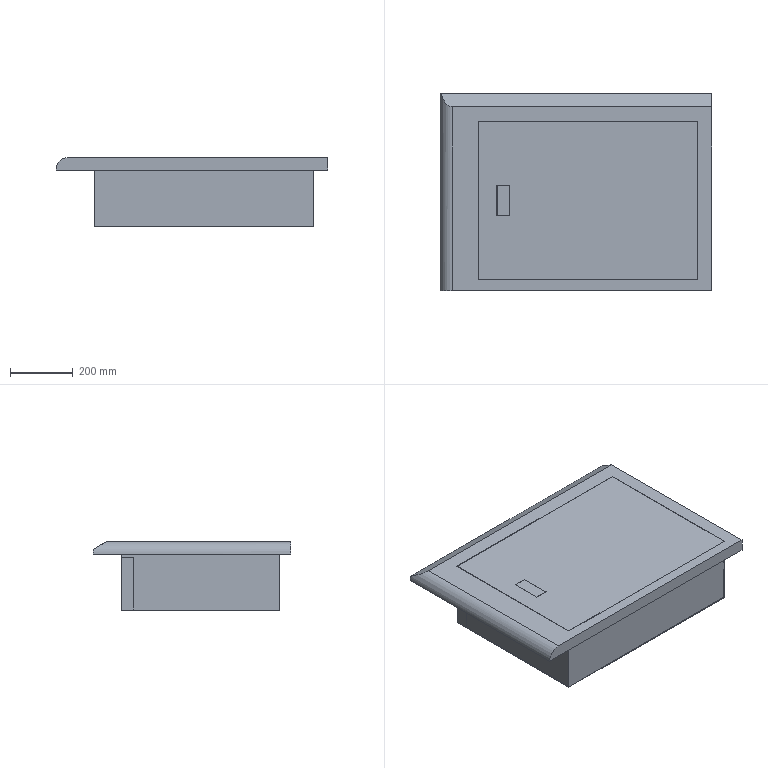Part | SolidWorks | features ICE 9, CutThin 1, Extrusion 1, Fillet 1, Shell 1 | 1 solid | 46 faces | box 867.5 x 630 x 220 mm | volume 27389806 mm3 | plane 45 | cylinder 1 | commonest cylinder face diameters 80 x1
STEP:
#1=CARTESIAN_POINT('',(-122.,595.,180.));
#2=VERTEX_POINT('',#1);
#3=CARTESIAN_POINT('',(-122.,-35.,180.));
#4=VERTEX_POINT('',#3);
#5=CARTESIAN_POINT('',(-122.,595.,180.));
#6=DIRECTION('',(0.,-1.,0.));
#7=VECTOR('',#6,1000.);
#8=LINE('',#5,#7);
#9=EDGE_CURVE('',#2,#4,#8,.T.);
#10=ORIENTED_EDGE('',*,*,#9,.F.);
#11=CARTESIAN_POINT('',(745.5,595.,180.));
#12=VERTEX_POINT('',#11);
#13=CARTESIAN_POINT('',(-122.,595.,180.));
#14=DIRECTION('',(-1.,0.,0.));
#15=VECTOR('',#14,1000.);
#16=LINE('',#13,#15);
#17=EDGE_CURVE('',#12,#2,#16,.T.);
#18=ORIENTED_EDGE('',*,*,#17,.F.);
#19=CARTESIAN_POINT('',(745.5,-35.,180.));
#20=VERTEX_POINT('',#19);
#21=CARTESIAN_POINT('',(745.5,595.,180.));
#22=DIRECTION('',(0.,1.,0.));
#23=VECTOR('',#22,1000.);
#24=LINE('',#21,#23);
#25=EDGE_CURVE('',#20,#12,#24,.T.);
#26=ORIENTED_EDGE('',*,*,#25,.F.);
#27=CARTESIAN_POINT('',(-122.,-35.,180.));
#28=DIRECTION('',(1.,0.,0.));
#29=VECTOR('',#28,1000.);
#30=LINE('',#27,#29);
#31=EDGE_CURVE('',#4,#20,#30,.T.);
#32=ORIENTED_EDGE('',*,*,#31,.F.);
#33=EDGE_LOOP('',(#10,#18,#26,#32));
#34=FACE_OUTER_BOUND('',#33,.T.);
#35=CARTESIAN_POINT('',(700.,505.,180.));
#36=VERTEX_POINT('',#35);
#37=CARTESIAN_POINT('',(0.,505.,180.));
#38=VERTEX_POINT('',#37);
#39=CARTESIAN_POINT('',(0.,505.,180.));
#40=DIRECTION('',(-1.,0.,0.));
#41=VECTOR('',#40,1000.);
#42=LINE('',#39,#41);
#43=EDGE_CURVE('',#36,#38,#42,.T.);
#44=ORIENTED_EDGE('',*,*,#43,.T.);
#45=CARTESIAN_POINT('',(0.,0.,180.));
#46=VERTEX_POINT('',#45);
#47=CARTESIAN_POINT('',(0.,0.,180.));
#48=DIRECTION('',(0.,-1.,0.));
#49=VECTOR('',#48,1000.);
#50=LINE('',#47,#49);
#51=EDGE_CURVE('',#38,#46,#50,.T.);
#52=ORIENTED_EDGE('',*,*,#51,.T.);
#53=CARTESIAN_POINT('',(700.,0.,180.));
#54=VERTEX_POINT('',#53);
#55=CARTESIAN_POINT('',(0.,0.,180.));
#56=DIRECTION('',(1.,0.,0.));
#57=VECTOR('',#56,1000.);
#58=LINE('',#55,#57);
#59=EDGE_CURVE('',#46,#54,#58,.T.);
#60=ORIENTED_EDGE('',*,*,#59,.T.);
#61=CARTESIAN_POINT('',(700.,0.,180.));
#62=DIRECTION('',(0.,1.,0.));
#63=VECTOR('',#62,1000.);
#64=LINE('',#61,#63);
#65=EDGE_CURVE('',#54,#36,#64,.T.);
#66=ORIENTED_EDGE('',*,*,#65,.T.);
#67=EDGE_LOOP('',(#44,#52,#60,#66));
#68=FACE_BOUND('',#67,.T.);
#69=CARTESIAN_POINT('',(0.,0.,180.));
#70=DIRECTION('',(0.,0.,1.));
#71=DIRECTION('',(1.,0.,0.));
#72=AXIS2_PLACEMENT_3D('',#69,#70,#71);
#73=PLANE('',#72);
#74=ADVANCED_FACE('',(#34,#68),#73,.F.);
#75=CARTESIAN_POINT('',(-82.,-35.,220.));
#76=VERTEX_POINT('',#75);
#77=CARTESIAN_POINT('',(745.5,-35.,220.));
#78=VERTEX_POINT('',#77);
#79=CARTESIAN_POINT('',(-122.,-35.,220.));
#80=DIRECTION('',(1.,0.,0.));
#81=VECTOR('',#80,1000.);
#82=LINE('',#79,#81);
#83=EDGE_CURVE('',#76,#78,#82,.T.);
#84=ORIENTED_EDGE('',*,*,#83,.F.);
#85=CARTESIAN_POINT('',(-82.,-35.,180.));
#86=DIRECTION('',(0.,-1.,0.));
#87=DIRECTION('',(0.,0.,1.));
#88=AXIS2_PLACEMENT_3D('',#85,#86,#87);
#89=CIRCLE('',#88,40.);
#90=EDGE_CURVE('',#76,#4,#89,.T.);
#91=ORIENTED_EDGE('',*,*,#90,.T.);
#92=ORIENTED_EDGE('',*,*,#31,.T.);
#93=CARTESIAN_POINT('',(745.5,-35.,220.));
#94=DIRECTION('',(0.,0.,-1.));
#95=VECTOR('',#94,1000.);
#96=LINE('',#93,#95);
#97=EDGE_CURVE('',#78,#20,#96,.T.);
#98=ORIENTED_EDGE('',*,*,#97,.F.);
#99=EDGE_LOOP('',(#84,#91,#92,#98));
#100=FACE_OUTER_BOUND('',#99,.T.);
#101=CARTESIAN_POINT('',(-122.,-35.,220.));
#102=DIRECTION('',(0.,1.,0.));
#103=DIRECTION('',(0.,0.,1.));
#104=AXIS2_PLACEMENT_3D('',#101,#102,#103);
#105=PLANE('',#104);
#106=ADVANCED_FACE('',(#100),#105,.F.);
#107=CARTESIAN_POINT('',(745.5,595.,195.));
#108=VERTEX_POINT('',#107);
#109=CARTESIAN_POINT('',(745.5,595.,220.));
#110=DIRECTION('',(0.,0.,-1.));
#111=VECTOR('',#110,1000.);
#112=LINE('',#109,#111);
#113=EDGE_CURVE('',#108,#12,#112,.T.);
#114=ORIENTED_EDGE('',*,*,#113,.F.);
#115=CARTESIAN_POINT('',(745.5,551.699,220.));
#116=VERTEX_POINT('',#115);
#117=CARTESIAN_POINT('',(745.5,595.,195.));
#118=DIRECTION('',(0.,-0.866,0.5));
#119=VECTOR('',#118,1000.);
#120=LINE('',#117,#119);
#121=EDGE_CURVE('',#108,#116,#120,.T.);
#122=ORIENTED_EDGE('',*,*,#121,.T.);
#123=CARTESIAN_POINT('',(745.5,595.,220.));
#124=DIRECTION('',(0.,1.,0.));
#125=VECTOR('',#124,1000.);
#126=LINE('',#123,#125);
#127=EDGE_CURVE('',#78,#116,#126,.T.);
#128=ORIENTED_EDGE('',*,*,#127,.F.);
#129=ORIENTED_EDGE('',*,*,#97,.T.);
#130=ORIENTED_EDGE('',*,*,#25,.T.);
#131=EDGE_LOOP('',(#114,#122,#128,#129,#130));
#132=FACE_OUTER_BOUND('',#131,.T.);
#133=CARTESIAN_POINT('',(745.5,595.,220.));
#134=DIRECTION('',(-1.,0.,0.));
#135=DIRECTION('',(0.,-1.,0.));
#136=AXIS2_PLACEMENT_3D('',#133,#134,#135);
#137=PLANE('',#136);
#138=ADVANCED_FACE('',(#132),#137,.F.);
#139=ORIENTED_EDGE('',*,*,#17,.T.);
#140=CARTESIAN_POINT('',(-119.081,595.,195.));
#141=VERTEX_POINT('',#140);
#142=CARTESIAN_POINT('',(-82.,595.,180.));
#143=DIRECTION('',(0.,1.,0.));
#144=DIRECTION('',(0.,0.,-1.));
#145=AXIS2_PLACEMENT_3D('',#142,#143,#144);
#146=CIRCLE('',#145,40.);
#147=EDGE_CURVE('',#2,#141,#146,.T.);
#148=ORIENTED_EDGE('',*,*,#147,.T.);
#149=CARTESIAN_POINT('',(745.5,595.,195.));
#150=DIRECTION('',(-1.,0.,0.));
#151=VECTOR('',#150,1000.);
#152=LINE('',#149,#151);
#153=EDGE_CURVE('',#108,#141,#152,.T.);
#154=ORIENTED_EDGE('',*,*,#153,.F.);
#155=ORIENTED_EDGE('',*,*,#113,.T.);
#156=EDGE_LOOP('',(#139,#148,#154,#155));
#157=FACE_OUTER_BOUND('',#156,.T.);
#158=CARTESIAN_POINT('',(-122.,595.,220.));
#159=DIRECTION('',(0.,-1.,0.));
#160=DIRECTION('',(0.,0.,-1.));
#161=AXIS2_PLACEMENT_3D('',#158,#159,#160);
#162=PLANE('',#161);
#163=ADVANCED_FACE('',(#157),#162,.F.);
#164=CARTESIAN_POINT('',(700.5,505.5,220.));
#165=VERTEX_POINT('',#164);
#166=CARTESIAN_POINT('',(-0.5,505.5,220.));
#167=VERTEX_POINT('',#166);
#168=CARTESIAN_POINT('',(700.,505.5,220.));
#169=DIRECTION('',(-1.,0.,0.));
#170=VECTOR('',#169,1000.);
#171=LINE('',#168,#170);
#172=EDGE_CURVE('',#165,#167,#171,.T.);
#173=ORIENTED_EDGE('',*,*,#172,.F.);
#174=CARTESIAN_POINT('',(700.5,-0.5,220.));
#175=VERTEX_POINT('',#174);
#176=CARTESIAN_POINT('',(700.5,0.,220.));
#177=DIRECTION('',(0.,1.,0.));
#178=VECTOR('',#177,1000.);
#179=LINE('',#176,#178);
#180=EDGE_CURVE('',#175,#165,#179,.T.);
#181=ORIENTED_EDGE('',*,*,#180,.F.);
#182=CARTESIAN_POINT('',(-0.5,-0.5,220.));
#183=VERTEX_POINT('',#182);
#184=CARTESIAN_POINT('',(0.,-0.5,220.));
#185=DIRECTION('',(1.,0.,0.));
#186=VECTOR('',#185,1000.);
#187=LINE('',#184,#186);
#188=EDGE_CURVE('',#183,#175,#187,.T.);
#189=ORIENTED_EDGE('',*,*,#188,.F.);
#190=CARTESIAN_POINT('',(-0.5,505.,220.));
#191=DIRECTION('',(0.,-1.,0.));
#192=VECTOR('',#191,1000.);
#193=LINE('',#190,#192);
#194=EDGE_CURVE('',#167,#183,#193,.T.);
#195=ORIENTED_EDGE('',*,*,#194,.F.);
#196=EDGE_LOOP('',(#173,#181,#189,#195));
#197=FACE_BOUND('',#196,.T.);
#198=CARTESIAN_POINT('',(-82.,551.699,220.));
#199=VERTEX_POINT('',#198);
#200=CARTESIAN_POINT('',(745.5,551.699,220.));
#201=DIRECTION('',(-1.,0.,0.));
#202=VECTOR('',#201,1000.);
#203=LINE('',#200,#202);
#204=EDGE_CURVE('',#116,#199,#203,.T.);
#205=ORIENTED_EDGE('',*,*,#204,.T.);
#206=CARTESIAN_POINT('',(-82.,-35.,220.));
#207=DIRECTION('',(0.,-1.,0.));
#208=VECTOR('',#207,1000.);
#209=LINE('',#206,#208);
#210=EDGE_CURVE('',#199,#76,#209,.T.);
#211=ORIENTED_EDGE('',*,*,#210,.T.);
#212=ORIENTED_EDGE('',*,*,#83,.T.);
#213=ORIENTED_EDGE('',*,*,#127,.T.);
#214=EDGE_LOOP('',(#205,#211,#212,#213));
#215=FACE_OUTER_BOUND('',#214,.T.);
#216=CARTESIAN_POINT('',(0.,0.,220.));
#217=DIRECTION('',(0.,0.,1.));
#218=DIRECTION('',(1.,0.,0.));
#219=AXIS2_PLACEMENT_3D('',#216,#217,#218);
#220=PLANE('',#219);
#221=ADVANCED_FACE('',(#197,#215),#220,.T.);
#222=CARTESIAN_POINT('',(0.,505.,0.));
#223=VERTEX_POINT('',#222);
#224=CARTESIAN_POINT('',(0.,0.,0.));
#225=VERTEX_POINT('',#224);
#226=CARTESIAN_POINT('',(0.,0.,0.));
#227=DIRECTION('',(0.,-1.,0.));
#228=VECTOR('',#227,1000.);
#229=LINE('',#226,#228);
#230=EDGE_CURVE('',#223,#225,#229,.T.);
#231=ORIENTED_EDGE('',*,*,#230,.F.);
#232=CARTESIAN_POINT('',(700.,505.,0.));
#233=VERTEX_POINT('',#232);
#234=CARTESIAN_POINT('',(700.,505.,0.));
#235=DIRECTION('',(-1.,0.,0.));
#236=VECTOR('',#235,1000.);
#237=LINE('',#234,#236);
#238=EDGE_CURVE('',#233,#223,#237,.T.);
#239=ORIENTED_EDGE('',*,*,#238,.F.);
#240=CARTESIAN_POINT('',(700.,0.,0.));
#241=VERTEX_POINT('',#240);
#242=CARTESIAN_POINT('',(700.,0.,0.));
#243=DIRECTION('',(0.,1.,0.));
#244=VECTOR('',#243,1000.);
#245=LINE('',#242,#244);
#246=EDGE_CURVE('',#241,#233,#245,.T.);
#247=ORIENTED_EDGE('',*,*,#246,.F.);
#248=CARTESIAN_POINT('',(0.,0.,0.));
#249=DIRECTION('',(1.,0.,0.));
#250=VECTOR('',#249,1000.);
#251=LINE('',#248,#250);
#252=EDGE_CURVE('',#225,#241,#251,.T.);
#253=ORIENTED_EDGE('',*,*,#252,.F.);
#254=EDGE_LOOP('',(#231,#239,#247,#253));
#255=FACE_OUTER_BOUND('',#254,.T.);
#256=CARTESIAN_POINT('',(0.,0.,0.));
#257=DIRECTION('',(0.,0.,-1.));
#258=DIRECTION('',(-1.,0.,0.));
#259=AXIS2_PLACEMENT_3D('',#256,#257,#258);
#260=PLANE('',#259);
#261=ADVANCED_FACE('',(#255),#260,.T.);
#262=CARTESIAN_POINT('',(700.,505.,180.));
#263=DIRECTION('',(0.,0.,-1.));
#264=VECTOR('',#263,1000.);
#265=LINE('',#262,#264);
#266=EDGE_CURVE('',#36,#233,#265,.T.);
#267=ORIENTED_EDGE('',*,*,#266,.T.);
#268=ORIENTED_EDGE('',*,*,#238,.T.);
#269=CARTESIAN_POINT('',(0.,505.,180.));
#270=DIRECTION('',(0.,0.,-1.));
#271=VECTOR('',#270,1000.);
#272=LINE('',#269,#271);
#273=EDGE_CURVE('',#38,#223,#272,.T.);
#274=ORIENTED_EDGE('',*,*,#273,.F.);
#275=ORIENTED_EDGE('',*,*,#43,.F.);
#276=EDGE_LOOP('',(#267,#268,#274,#275));
#277=FACE_OUTER_BOUND('',#276,.T.);
#278=CARTESIAN_POINT('',(0.,505.,180.));
#279=DIRECTION('',(0.,-1.,0.));
#280=DIRECTION('',(0.,0.,-1.));
#281=AXIS2_PLACEMENT_3D('',#278,#279,#280);
#282=PLANE('',#281);
#283=ADVANCED_FACE('',(#277),#282,.F.);
#284=ORIENTED_EDGE('',*,*,#246,.T.);
#285=ORIENTED_EDGE('',*,*,#266,.F.);
#286=ORIENTED_EDGE('',*,*,#65,.F.);
#287=CARTESIAN_POINT('',(700.,0.,180.));
#288=DIRECTION('',(0.,0.,-1.));
#289=VECTOR('',#288,1000.);
#290=LINE('',#287,#289);
#291=EDGE_CURVE('',#54,#241,#290,.T.);
#292=ORIENTED_EDGE('',*,*,#291,.T.);
#293=EDGE_LOOP('',(#284,#285,#286,#292));
#294=FACE_OUTER_BOUND('',#293,.T.);
#295=CARTESIAN_POINT('',(700.,0.,180.));
#296=DIRECTION('',(-1.,0.,0.));
#297=DIRECTION('',(0.,0.,1.));
#298=AXIS2_PLACEMENT_3D('',#295,#296,#297);
#299=PLANE('',#298);
#300=ADVANCED_FACE('',(#294),#299,.F.);
#301=CARTESIAN_POINT('',(0.,0.,180.));
#302=DIRECTION('',(0.,0.,-1.));
#303=VECTOR('',#302,1000.);
#304=LINE('',#301,#303);
#305=EDGE_CURVE('',#46,#225,#304,.T.);
#306=ORIENTED_EDGE('',*,*,#305,.T.);
#307=ORIENTED_EDGE('',*,*,#252,.T.);
#308=ORIENTED_EDGE('',*,*,#291,.F.);
#309=ORIENTED_EDGE('',*,*,#59,.F.);
#310=EDGE_LOOP('',(#306,#307,#308,#309));
#311=FACE_OUTER_BOUND('',#310,.T.);
#312=CARTESIAN_POINT('',(0.,0.,180.));
#313=DIRECTION('',(0.,1.,0.));
#314=DIRECTION('',(0.,0.,1.));
#315=AXIS2_PLACEMENT_3D('',#312,#313,#314);
#316=PLANE('',#315);
#317=ADVANCED_FACE('',(#311),#316,.F.);
#318=ORIENTED_EDGE('',*,*,#273,.T.);
#319=ORIENTED_EDGE('',*,*,#230,.T.);
#320=ORIENTED_EDGE('',*,*,#305,.F.);
#321=ORIENTED_EDGE('',*,*,#51,.F.);
#322=EDGE_LOOP('',(#318,#319,#320,#321));
#323=FACE_OUTER_BOUND('',#322,.T.);
#324=CARTESIAN_POINT('',(0.,0.,180.));
#325=DIRECTION('',(1.,0.,0.));
#326=DIRECTION('',(0.,0.,-1.));
#327=AXIS2_PLACEMENT_3D('',#324,#325,#326);
#328=PLANE('',#327);
#329=ADVANCED_FACE('',(#323),#328,.F.);
#330=ORIENTED_EDGE('',*,*,#153,.T.);
#331=CARTESIAN_POINT('',(-119.081,595.,195.));
#332=CARTESIAN_POINT('',(-112.772,567.988,210.596));
#333=CARTESIAN_POINT('',(-98.823,551.699,220.));
#334=CARTESIAN_POINT('',(-82.,551.699,220.));
#335=(BOUNDED_CURVE()B_SPLINE_CURVE(3,(#331,#332,#333,#334),.UNSPECIFIED.,.F.,.T.)B_SPLINE_CURVE_WITH_KNOTS((4,4),(1.955,3.142),.UNSPECIFIED.)CURVE()GEOMETRIC_REPRESENTATION_ITEM()RATIONAL_B_SPLINE_CURVE((1.,0.8861,0.8861,1.))REPRESENTATION_ITEM(''));
#336=EDGE_CURVE('',#141,#199,#335,.T.);
#337=ORIENTED_EDGE('',*,*,#336,.T.);
#338=ORIENTED_EDGE('',*,*,#204,.F.);
#339=ORIENTED_EDGE('',*,*,#121,.F.);
#340=EDGE_LOOP('',(#330,#337,#338,#339));
#341=FACE_OUTER_BOUND('',#340,.T.);
#342=CARTESIAN_POINT('',(745.5,595.,195.));
#343=DIRECTION('',(0.,-0.5,-0.866));
#344=DIRECTION('',(0.,0.866,-0.5));
#345=AXIS2_PLACEMENT_3D('',#342,#343,#344);
#346=PLANE('',#345);
#347=ADVANCED_FACE('',(#341),#346,.F.);
#348=ORIENTED_EDGE('',*,*,#147,.F.);
#349=ORIENTED_EDGE('',*,*,#9,.T.);
#350=ORIENTED_EDGE('',*,*,#90,.F.);
#351=ORIENTED_EDGE('',*,*,#210,.F.);
#352=ORIENTED_EDGE('',*,*,#336,.F.);
#353=EDGE_LOOP('',(#348,#349,#350,#351,#352));
#354=FACE_OUTER_BOUND('',#353,.T.);
#355=CARTESIAN_POINT('',(-82.,0.,180.));
#356=DIRECTION('',(0.,1.,0.));
#357=DIRECTION('',(-1.,0.,0.));
#358=AXIS2_PLACEMENT_3D('',#355,#356,#357);
#359=CYLINDRICAL_SURFACE('',#358,40.);
#360=ADVANCED_FACE('',(#354),#359,.T.);
#361=ORIENTED_EDGE('',*,*,#172,.T.);
#362=CARTESIAN_POINT('',(-0.5,505.5,210.));
#363=VERTEX_POINT('',#362);
#364=CARTESIAN_POINT('',(-0.5,505.5,210.));
#365=DIRECTION('',(0.,0.,1.));
#366=VECTOR('',#365,1000.);
#367=LINE('',#364,#366);
#368=EDGE_CURVE('',#363,#167,#367,.T.);
#369=ORIENTED_EDGE('',*,*,#368,.F.);
#370=CARTESIAN_POINT('',(700.5,505.5,210.));
#371=VERTEX_POINT('',#370);
#372=CARTESIAN_POINT('',(700.,505.5,210.));
#373=DIRECTION('',(-1.,0.,0.));
#374=VECTOR('',#373,1000.);
#375=LINE('',#372,#374);
#376=EDGE_CURVE('',#371,#363,#375,.T.);
#377=ORIENTED_EDGE('',*,*,#376,.F.);
#378=CARTESIAN_POINT('',(700.5,505.5,210.));
#379=DIRECTION('',(0.,0.,1.));
#380=VECTOR('',#379,1000.);
#381=LINE('',#378,#380);
#382=EDGE_CURVE('',#371,#165,#381,.T.);
#383=ORIENTED_EDGE('',*,*,#382,.T.);
#384=EDGE_LOOP('',(#361,#369,#377,#383));
#385=FACE_OUTER_BOUND('',#384,.T.);
#386=CARTESIAN_POINT('',(700.,505.5,210.));
#387=DIRECTION('',(0.,1.,0.));
#388=DIRECTION('',(0.,0.,1.));
#389=AXIS2_PLACEMENT_3D('',#386,#387,#388);
#390=PLANE('',#389);
#391=ADVANCED_FACE('',(#385),#390,.F.);
#392=ORIENTED_EDGE('',*,*,#180,.T.);
#393=ORIENTED_EDGE('',*,*,#382,.F.);
#394=CARTESIAN_POINT('',(700.5,-0.5,210.));
#395=VERTEX_POINT('',#394);
#396=CARTESIAN_POINT('',(700.5,0.,210.));
#397=DIRECTION('',(0.,1.,0.));
#398=VECTOR('',#397,1000.);
#399=LINE('',#396,#398);
#400=EDGE_CURVE('',#395,#371,#399,.T.);
#401=ORIENTED_EDGE('',*,*,#400,.F.);
#402=CARTESIAN_POINT('',(700.5,-0.5,210.));
#403=DIRECTION('',(0.,0.,1.));
#404=VECTOR('',#403,1000.);
#405=LINE('',#402,#404);
#406=EDGE_CURVE('',#395,#175,#405,.T.);
#407=ORIENTED_EDGE('',*,*,#406,.T.);
#408=EDGE_LOOP('',(#392,#393,#401,#407));
#409=FACE_OUTER_BOUND('',#408,.T.);
#410=CARTESIAN_POINT('',(700.5,0.,210.));
#411=DIRECTION('',(1.,0.,0.));
#412=DIRECTION('',(0.,0.,-1.));
#413=AXIS2_PLACEMENT_3D('',#410,#411,#412);
#414=PLANE('',#413);
#415=ADVANCED_FACE('',(#409),#414,.F.);
#416=ORIENTED_EDGE('',*,*,#188,.T.);
#417=ORIENTED_EDGE('',*,*,#406,.F.);
#418=CARTESIAN_POINT('',(-0.5,-0.5,210.));
#419=VERTEX_POINT('',#418);
#420=CARTESIAN_POINT('',(0.,-0.5,210.));
#421=DIRECTION('',(1.,0.,0.));
#422=VECTOR('',#421,1000.);
#423=LINE('',#420,#422);
#424=EDGE_CURVE('',#419,#395,#423,.T.);
#425=ORIENTED_EDGE('',*,*,#424,.F.);
#426=CARTESIAN_POINT('',(-0.5,-0.5,210.));
#427=DIRECTION('',(0.,0.,1.));
#428=VECTOR('',#427,1000.);
#429=LINE('',#426,#428);
#430=EDGE_CURVE('',#419,#183,#429,.T.);
#431=ORIENTED_EDGE('',*,*,#430,.T.);
#432=EDGE_LOOP('',(#416,#417,#425,#431));
#433=FACE_OUTER_BOUND('',#432,.T.);
#434=CARTESIAN_POINT('',(0.,-0.5,210.));
#435=DIRECTION('',(0.,-1.,0.));
#436=DIRECTION('',(0.,0.,-1.));
#437=AXIS2_PLACEMENT_3D('',#434,#435,#436);
#438=PLANE('',#437);
#439=ADVANCED_FACE('',(#433),#438,.F.);
#440=ORIENTED_EDGE('',*,*,#194,.T.);
#441=ORIENTED_EDGE('',*,*,#430,.F.);
#442=CARTESIAN_POINT('',(-0.5,505.,210.));
#443=DIRECTION('',(0.,-1.,0.));
#444=VECTOR('',#443,1000.);
#445=LINE('',#442,#444);
#446=EDGE_CURVE('',#363,#419,#445,.T.);
#447=ORIENTED_EDGE('',*,*,#446,.F.);
#448=ORIENTED_EDGE('',*,*,#368,.T.);
#449=EDGE_LOOP('',(#440,#441,#447,#448));
#450=FACE_OUTER_BOUND('',#449,.T.);
#451=CARTESIAN_POINT('',(-0.5,505.,210.));
#452=DIRECTION('',(-1.,0.,0.));
#453=DIRECTION('',(0.,0.,1.));
#454=AXIS2_PLACEMENT_3D('',#451,#452,#453);
#455=PLANE('',#454);
#456=ADVANCED_FACE('',(#450),#455,.F.);
#457=CARTESIAN_POINT('',(700.,0.,210.));
#458=VERTEX_POINT('',#457);
#459=CARTESIAN_POINT('',(700.,505.,210.));
#460=VERTEX_POINT('',#459);
#461=CARTESIAN_POINT('',(700.,0.,210.));
#462=DIRECTION('',(0.,1.,0.));
#463=VECTOR('',#462,1000.);
#464=LINE('',#461,#463);
#465=EDGE_CURVE('',#458,#460,#464,.T.);
#466=ORIENTED_EDGE('',*,*,#465,.F.);
#467=CARTESIAN_POINT('',(0.,0.,210.));
#468=VERTEX_POINT('',#467);
#469=CARTESIAN_POINT('',(0.,0.,210.));
#470=DIRECTION('',(1.,0.,0.));
#471=VECTOR('',#470,1000.);
#472=LINE('',#469,#471);
#473=EDGE_CURVE('',#468,#458,#472,.T.);
#474=ORIENTED_EDGE('',*,*,#473,.F.);
#475=CARTESIAN_POINT('',(0.,505.,210.));
#476=VERTEX_POINT('',#475);
#477=CARTESIAN_POINT('',(0.,505.,210.));
#478=DIRECTION('',(0.,-1.,0.));
#479=VECTOR('',#478,1000.);
#480=LINE('',#477,#479);
#481=EDGE_CURVE('',#476,#468,#480,.T.);
#482=ORIENTED_EDGE('',*,*,#481,.F.);
#483=CARTESIAN_POINT('',(700.,505.,210.));
#484=DIRECTION('',(-1.,0.,0.));
#485=VECTOR('',#484,1000.);
#486=LINE('',#483,#485);
#487=EDGE_CURVE('',#460,#476,#486,.T.);
#488=ORIENTED_EDGE('',*,*,#487,.F.);
#489=EDGE_LOOP('',(#466,#474,#482,#488));
#490=FACE_BOUND('',#489,.T.);
#491=ORIENTED_EDGE('',*,*,#376,.T.);
#492=ORIENTED_EDGE('',*,*,#446,.T.);
#493=ORIENTED_EDGE('',*,*,#424,.T.);
#494=ORIENTED_EDGE('',*,*,#400,.T.);
#495=EDGE_LOOP('',(#491,#492,#493,#494));
#496=FACE_OUTER_BOUND('',#495,.T.);
#497=CARTESIAN_POINT('',(0.,0.,210.));
#498=DIRECTION('',(0.,0.,1.));
#499=DIRECTION('',(1.,0.,0.));
#500=AXIS2_PLACEMENT_3D('',#497,#498,#499);
#501=PLANE('',#500);
#502=ADVANCED_FACE('',(#490,#496),#501,.T.);
#503=CARTESIAN_POINT('',(700.,505.,220.));
#504=VERTEX_POINT('',#503);
#505=CARTESIAN_POINT('',(0.,505.,220.));
#506=VERTEX_POINT('',#505);
#507=CARTESIAN_POINT('',(700.,505.,220.));
#508=DIRECTION('',(-1.,0.,0.));
#509=VECTOR('',#508,1000.);
#510=LINE('',#507,#509);
#511=EDGE_CURVE('',#504,#506,#510,.T.);
#512=ORIENTED_EDGE('',*,*,#511,.F.);
#513=CARTESIAN_POINT('',(700.,505.,210.));
#514=DIRECTION('',(0.,0.,1.));
#515=VECTOR('',#514,1000.);
#516=LINE('',#513,#515);
#517=EDGE_CURVE('',#460,#504,#516,.T.);
#518=ORIENTED_EDGE('',*,*,#517,.F.);
#519=ORIENTED_EDGE('',*,*,#487,.T.);
#520=CARTESIAN_POINT('',(0.,505.,210.));
#521=DIRECTION('',(0.,0.,1.));
#522=VECTOR('',#521,1000.);
#523=LINE('',#520,#522);
#524=EDGE_CURVE('',#476,#506,#523,.T.);
#525=ORIENTED_EDGE('',*,*,#524,.T.);
#526=EDGE_LOOP('',(#512,#518,#519,#525));
#527=FACE_OUTER_BOUND('',#526,.T.);
#528=CARTESIAN_POINT('',(700.,505.,210.));
#529=DIRECTION('',(0.,1.,0.));
#530=DIRECTION('',(0.,0.,1.));
#531=AXIS2_PLACEMENT_3D('',#528,#529,#530);
#532=PLANE('',#531);
#533=ADVANCED_FACE('',(#527),#532,.T.);
#534=CARTESIAN_POINT('',(700.,0.,220.));
#535=VERTEX_POINT('',#534);
#536=CARTESIAN_POINT('',(700.,0.,220.));
#537=DIRECTION('',(0.,1.,0.));
#538=VECTOR('',#537,1000.);
#539=LINE('',#536,#538);
#540=EDGE_CURVE('',#535,#504,#539,.T.);
#541=ORIENTED_EDGE('',*,*,#540,.F.);
#542=CARTESIAN_POINT('',(700.,0.,210.));
#543=DIRECTION('',(0.,0.,1.));
#544=VECTOR('',#543,1000.);
#545=LINE('',#542,#544);
#546=EDGE_CURVE('',#458,#535,#545,.T.);
#547=ORIENTED_EDGE('',*,*,#546,.F.);
#548=ORIENTED_EDGE('',*,*,#465,.T.);
#549=ORIENTED_EDGE('',*,*,#517,.T.);
#550=EDGE_LOOP('',(#541,#547,#548,#549));
#551=FACE_OUTER_BOUND('',#550,.T.);
#552=CARTESIAN_POINT('',(700.,0.,210.));
#553=DIRECTION('',(1.,0.,0.));
#554=DIRECTION('',(0.,0.,-1.));
#555=AXIS2_PLACEMENT_3D('',#552,#553,#554);
#556=PLANE('',#555);
#557=ADVANCED_FACE('',(#551),#556,.T.);
#558=CARTESIAN_POINT('',(0.,0.,220.));
#559=VERTEX_POINT('',#558);
#560=CARTESIAN_POINT('',(0.,0.,220.));
#561=DIRECTION('',(1.,0.,0.));
#562=VECTOR('',#561,1000.);
#563=LINE('',#560,#562);
#564=EDGE_CURVE('',#559,#535,#563,.T.);
#565=ORIENTED_EDGE('',*,*,#564,.F.);
#566=CARTESIAN_POINT('',(0.,0.,210.));
#567=DIRECTION('',(0.,0.,1.));
#568=VECTOR('',#567,1000.);
#569=LINE('',#566,#568);
#570=EDGE_CURVE('',#468,#559,#569,.T.);
#571=ORIENTED_EDGE('',*,*,#570,.F.);
#572=ORIENTED_EDGE('',*,*,#473,.T.);
#573=ORIENTED_EDGE('',*,*,#546,.T.);
#574=EDGE_LOOP('',(#565,#571,#572,#573));
#575=FACE_OUTER_BOUND('',#574,.T.);
#576=CARTESIAN_POINT('',(0.,0.,210.));
#577=DIRECTION('',(0.,-1.,0.));
#578=DIRECTION('',(0.,0.,-1.));
#579=AXIS2_PLACEMENT_3D('',#576,#577,#578);
#580=PLANE('',#579);
#581=ADVANCED_FACE('',(#575),#580,.T.);
#582=CARTESIAN_POINT('',(0.,505.,220.));
#583=DIRECTION('',(0.,-1.,0.));
#584=VECTOR('',#583,1000.);
#585=LINE('',#582,#584);
#586=EDGE_CURVE('',#506,#559,#585,.T.);
#587=ORIENTED_EDGE('',*,*,#586,.F.);
#588=ORIENTED_EDGE('',*,*,#524,.F.);
#589=ORIENTED_EDGE('',*,*,#481,.T.);
#590=ORIENTED_EDGE('',*,*,#570,.T.);
#591=EDGE_LOOP('',(#587,#588,#589,#590));
#592=FACE_OUTER_BOUND('',#591,.T.);
#593=CARTESIAN_POINT('',(0.,505.,210.));
#594=DIRECTION('',(-1.,0.,0.));
#595=DIRECTION('',(0.,0.,1.));
#596=AXIS2_PLACEMENT_3D('',#593,#594,#595);
#597=PLANE('',#596);
#598=ADVANCED_FACE('',(#592),#597,.T.);
#599=CARTESIAN_POINT('',(59.5,301.,220.));
#600=VERTEX_POINT('',#599);
#601=CARTESIAN_POINT('',(59.5,204.,220.));
#602=VERTEX_POINT('',#601);
#603=CARTESIAN_POINT('',(59.5,300.5,220.));
#604=DIRECTION('',(0.,-1.,0.));
#605=VECTOR('',#604,1000.);
#606=LINE('',#603,#605);
#607=EDGE_CURVE('',#600,#602,#606,.T.);
#608=ORIENTED_EDGE('',*,*,#607,.F.);
#609=CARTESIAN_POINT('',(100.5,301.,220.));
#610=VERTEX_POINT('',#609);
#611=CARTESIAN_POINT('',(60.,301.,220.));
#612=DIRECTION('',(-1.,0.,0.));
#613=VECTOR('',#612,1000.);
#614=LINE('',#611,#613);
#615=EDGE_CURVE('',#610,#600,#614,.T.);
#616=ORIENTED_EDGE('',*,*,#615,.F.);
#617=CARTESIAN_POINT('',(100.5,204.,220.));
#618=VERTEX_POINT('',#617);
#619=CARTESIAN_POINT('',(100.5,300.5,220.));
#620=DIRECTION('',(0.,1.,0.));
#621=VECTOR('',#620,1000.);
#622=LINE('',#619,#621);
#623=EDGE_CURVE('',#618,#610,#622,.T.);
#624=ORIENTED_EDGE('',*,*,#623,.F.);
#625=CARTESIAN_POINT('',(60.,204.,220.));
#626=DIRECTION('',(1.,0.,0.));
#627=VECTOR('',#626,1000.);
#628=LINE('',#625,#627);
#629=EDGE_CURVE('',#602,#618,#628,.T.);
#630=ORIENTED_EDGE('',*,*,#629,.F.);
#631=EDGE_LOOP('',(#608,#616,#624,#630));
#632=FACE_BOUND('',#631,.T.);
#633=ORIENTED_EDGE('',*,*,#540,.T.);
#634=ORIENTED_EDGE('',*,*,#511,.T.);
#635=ORIENTED_EDGE('',*,*,#586,.T.);
#636=ORIENTED_EDGE('',*,*,#564,.T.);
#637=EDGE_LOOP('',(#633,#634,#635,#636));
#638=FACE_OUTER_BOUND('',#637,.T.);
#639=CARTESIAN_POINT('',(0.,0.,220.));
#640=DIRECTION('',(0.,0.,1.));
#641=DIRECTION('',(1.,0.,0.));
#642=AXIS2_PLACEMENT_3D('',#639,#640,#641);
#643=PLANE('',#642);
#644=ADVANCED_FACE('',(#632,#638),#643,.T.);
#645=ORIENTED_EDGE('',*,*,#607,.T.);
#646=CARTESIAN_POINT('',(59.5,204.,210.));
#647=VERTEX_POINT('',#646);
#648=CARTESIAN_POINT('',(59.5,204.,210.));
#649=DIRECTION('',(0.,0.,1.));
#650=VECTOR('',#649,1000.);
#651=LINE('',#648,#650);
#652=EDGE_CURVE('',#647,#602,#651,.T.);
#653=ORIENTED_EDGE('',*,*,#652,.F.);
#654=CARTESIAN_POINT('',(59.5,301.,210.));
#655=VERTEX_POINT('',#654);
#656=CARTESIAN_POINT('',(59.5,300.5,210.));
#657=DIRECTION('',(0.,-1.,0.));
#658=VECTOR('',#657,1000.);
#659=LINE('',#656,#658);
#660=EDGE_CURVE('',#655,#647,#659,.T.);
#661=ORIENTED_EDGE('',*,*,#660,.F.);
#662=CARTESIAN_POINT('',(59.5,301.,210.));
#663=DIRECTION('',(0.,0.,1.));
#664=VECTOR('',#663,1000.);
#665=LINE('',#662,#664);
#666=EDGE_CURVE('',#655,#600,#665,.T.);
#667=ORIENTED_EDGE('',*,*,#666,.T.);
#668=EDGE_LOOP('',(#645,#653,#661,#667));
#669=FACE_OUTER_BOUND('',#668,.T.);
#670=CARTESIAN_POINT('',(59.5,300.5,210.));
#671=DIRECTION('',(-1.,0.,0.));
#672=DIRECTION('',(0.,0.,1.));
#673=AXIS2_PLACEMENT_3D('',#670,#671,#672);
#674=PLANE('',#673);
#675=ADVANCED_FACE('',(#669),#674,.F.);
#676=ORIENTED_EDGE('',*,*,#615,.T.);
#677=ORIENTED_EDGE('',*,*,#666,.F.);
#678=CARTESIAN_POINT('',(100.5,301.,210.));
#679=VERTEX_POINT('',#678);
#680=CARTESIAN_POINT('',(60.,301.,210.));
#681=DIRECTION('',(-1.,0.,0.));
#682=VECTOR('',#681,1000.);
#683=LINE('',#680,#682);
#684=EDGE_CURVE('',#679,#655,#683,.T.);
#685=ORIENTED_EDGE('',*,*,#684,.F.);
#686=CARTESIAN_POINT('',(100.5,301.,210.));
#687=DIRECTION('',(0.,0.,1.));
#688=VECTOR('',#687,1000.);
#689=LINE('',#686,#688);
#690=EDGE_CURVE('',#679,#610,#689,.T.);
#691=ORIENTED_EDGE('',*,*,#690,.T.);
#692=EDGE_LOOP('',(#676,#677,#685,#691));
#693=FACE_OUTER_BOUND('',#692,.T.);
#694=CARTESIAN_POINT('',(60.,301.,210.));
#695=DIRECTION('',(0.,1.,0.));
#696=DIRECTION('',(0.,0.,1.));
#697=AXIS2_PLACEMENT_3D('',#694,#695,#696);
#698=PLANE('',#697);
#699=ADVANCED_FACE('',(#693),#698,.F.);
#700=ORIENTED_EDGE('',*,*,#623,.T.);
#701=ORIENTED_EDGE('',*,*,#690,.F.);
#702=CARTESIAN_POINT('',(100.5,204.,210.));
#703=VERTEX_POINT('',#702);
#704=CARTESIAN_POINT('',(100.5,300.5,210.));
#705=DIRECTION('',(0.,1.,0.));
#706=VECTOR('',#705,1000.);
#707=LINE('',#704,#706);
#708=EDGE_CURVE('',#703,#679,#707,.T.);
#709=ORIENTED_EDGE('',*,*,#708,.F.);
#710=CARTESIAN_POINT('',(100.5,204.,210.));
#711=DIRECTION('',(0.,0.,1.));
#712=VECTOR('',#711,1000.);
#713=LINE('',#710,#712);
#714=EDGE_CURVE('',#703,#618,#713,.T.);
#715=ORIENTED_EDGE('',*,*,#714,.T.);
#716=EDGE_LOOP('',(#700,#701,#709,#715));
#717=FACE_OUTER_BOUND('',#716,.T.);
#718=CARTESIAN_POINT('',(100.5,300.5,210.));
#719=DIRECTION('',(1.,0.,0.));
#720=DIRECTION('',(0.,0.,-1.));
#721=AXIS2_PLACEMENT_3D('',#718,#719,#720);
#722=PLANE('',#721);
#723=ADVANCED_FACE('',(#717),#722,.F.);
#724=ORIENTED_EDGE('',*,*,#629,.T.);
#725=ORIENTED_EDGE('',*,*,#714,.F.);
#726=CARTESIAN_POINT('',(60.,204.,210.));
#727=DIRECTION('',(1.,0.,0.));
#728=VECTOR('',#727,1000.);
#729=LINE('',#726,#728);
#730=EDGE_CURVE('',#647,#703,#729,.T.);
#731=ORIENTED_EDGE('',*,*,#730,.F.);
#732=ORIENTED_EDGE('',*,*,#652,.T.);
#733=EDGE_LOOP('',(#724,#725,#731,#732));
#734=FACE_OUTER_BOUND('',#733,.T.);
#735=CARTESIAN_POINT('',(60.,204.,210.));
#736=DIRECTION('',(0.,-1.,0.));
#737=DIRECTION('',(0.,0.,-1.));
#738=AXIS2_PLACEMENT_3D('',#735,#736,#737);
#739=PLANE('',#738);
#740=ADVANCED_FACE('',(#734),#739,.F.);
#741=CARTESIAN_POINT('',(100.,300.5,210.));
#742=VERTEX_POINT('',#741);
#743=CARTESIAN_POINT('',(60.,300.5,210.));
#744=VERTEX_POINT('',#743);
#745=CARTESIAN_POINT('',(60.,300.5,210.));
#746=DIRECTION('',(-1.,0.,0.));
#747=VECTOR('',#746,1000.);
#748=LINE('',#745,#747);
#749=EDGE_CURVE('',#742,#744,#748,.T.);
#750=ORIENTED_EDGE('',*,*,#749,.F.);
#751=CARTESIAN_POINT('',(100.,204.5,210.));
#752=VERTEX_POINT('',#751);
#753=CARTESIAN_POINT('',(100.,300.5,210.));
#754=DIRECTION('',(0.,1.,0.));
#755=VECTOR('',#754,1000.);
#756=LINE('',#753,#755);
#757=EDGE_CURVE('',#752,#742,#756,.T.);
#758=ORIENTED_EDGE('',*,*,#757,.F.);
#759=CARTESIAN_POINT('',(60.,204.5,210.));
#760=VERTEX_POINT('',#759);
#761=CARTESIAN_POINT('',(60.,204.5,210.));
#762=DIRECTION('',(1.,0.,0.));
#763=VECTOR('',#762,1000.);
#764=LINE('',#761,#763);
#765=EDGE_CURVE('',#760,#752,#764,.T.);
#766=ORIENTED_EDGE('',*,*,#765,.F.);
#767=CARTESIAN_POINT('',(60.,300.5,210.));
#768=DIRECTION('',(0.,-1.,0.));
#769=VECTOR('',#768,1000.);
#770=LINE('',#767,#769);
#771=EDGE_CURVE('',#744,#760,#770,.T.);
#772=ORIENTED_EDGE('',*,*,#771,.F.);
#773=EDGE_LOOP('',(#750,#758,#766,#772));
#774=FACE_BOUND('',#773,.T.);
#775=ORIENTED_EDGE('',*,*,#660,.T.);
#776=ORIENTED_EDGE('',*,*,#730,.T.);
#777=ORIENTED_EDGE('',*,*,#708,.T.);
#778=ORIENTED_EDGE('',*,*,#684,.T.);
#779=EDGE_LOOP('',(#775,#776,#777,#778));
#780=FACE_OUTER_BOUND('',#779,.T.);
#781=CARTESIAN_POINT('',(0.,0.,210.));
#782=DIRECTION('',(0.,0.,1.));
#783=DIRECTION('',(1.,0.,0.));
#784=AXIS2_PLACEMENT_3D('',#781,#782,#783);
#785=PLANE('',#784);
#786=ADVANCED_FACE('',(#774,#780),#785,.T.);
#787=CARTESIAN_POINT('',(60.,300.5,220.));
#788=VERTEX_POINT('',#787);
#789=CARTESIAN_POINT('',(60.,204.5,220.));
#790=VERTEX_POINT('',#789);
#791=CARTESIAN_POINT('',(60.,300.5,220.));
#792=DIRECTION('',(0.,-1.,0.));
#793=VECTOR('',#792,1000.);
#794=LINE('',#791,#793);
#795=EDGE_CURVE('',#788,#790,#794,.T.);
#796=ORIENTED_EDGE('',*,*,#795,.F.);
#797=CARTESIAN_POINT('',(60.,300.5,210.));
#798=DIRECTION('',(0.,0.,1.));
#799=VECTOR('',#798,1000.);
#800=LINE('',#797,#799);
#801=EDGE_CURVE('',#744,#788,#800,.T.);
#802=ORIENTED_EDGE('',*,*,#801,.F.);
#803=ORIENTED_EDGE('',*,*,#771,.T.);
#804=CARTESIAN_POINT('',(60.,204.5,210.));
#805=DIRECTION('',(0.,0.,1.));
#806=VECTOR('',#805,1000.);
#807=LINE('',#804,#806);
#808=EDGE_CURVE('',#760,#790,#807,.T.);
#809=ORIENTED_EDGE('',*,*,#808,.T.);
#810=EDGE_LOOP('',(#796,#802,#803,#809));
#811=FACE_OUTER_BOUND('',#810,.T.);
#812=CARTESIAN_POINT('',(60.,300.5,210.));
#813=DIRECTION('',(-1.,0.,0.));
#814=DIRECTION('',(0.,0.,1.));
#815=AXIS2_PLACEMENT_3D('',#812,#813,#814);
#816=PLANE('',#815);
#817=ADVANCED_FACE('',(#811),#816,.T.);
#818=CARTESIAN_POINT('',(100.,300.5,220.));
#819=VERTEX_POINT('',#818);
#820=CARTESIAN_POINT('',(60.,300.5,220.));
#821=DIRECTION('',(-1.,0.,0.));
#822=VECTOR('',#821,1000.);
#823=LINE('',#820,#822);
#824=EDGE_CURVE('',#819,#788,#823,.T.);
#825=ORIENTED_EDGE('',*,*,#824,.F.);
#826=CARTESIAN_POINT('',(100.,300.5,210.));
#827=DIRECTION('',(0.,0.,1.));
#828=VECTOR('',#827,1000.);
#829=LINE('',#826,#828);
#830=EDGE_CURVE('',#742,#819,#829,.T.);
#831=ORIENTED_EDGE('',*,*,#830,.F.);
#832=ORIENTED_EDGE('',*,*,#749,.T.);
#833=ORIENTED_EDGE('',*,*,#801,.T.);
#834=EDGE_LOOP('',(#825,#831,#832,#833));
#835=FACE_OUTER_BOUND('',#834,.T.);
#836=CARTESIAN_POINT('',(60.,300.5,210.));
#837=DIRECTION('',(0.,1.,0.));
#838=DIRECTION('',(0.,0.,1.));
#839=AXIS2_PLACEMENT_3D('',#836,#837,#838);
#840=PLANE('',#839);
#841=ADVANCED_FACE('',(#835),#840,.T.);
#842=CARTESIAN_POINT('',(100.,204.5,220.));
#843=VERTEX_POINT('',#842);
#844=CARTESIAN_POINT('',(100.,300.5,220.));
#845=DIRECTION('',(0.,1.,0.));
#846=VECTOR('',#845,1000.);
#847=LINE('',#844,#846);
#848=EDGE_CURVE('',#843,#819,#847,.T.);
#849=ORIENTED_EDGE('',*,*,#848,.F.);
#850=CARTESIAN_POINT('',(100.,204.5,210.));
#851=DIRECTION('',(0.,0.,1.));
#852=VECTOR('',#851,1000.);
#853=LINE('',#850,#852);
#854=EDGE_CURVE('',#752,#843,#853,.T.);
#855=ORIENTED_EDGE('',*,*,#854,.F.);
#856=ORIENTED_EDGE('',*,*,#757,.T.);
#857=ORIENTED_EDGE('',*,*,#830,.T.);
#858=EDGE_LOOP('',(#849,#855,#856,#857));
#859=FACE_OUTER_BOUND('',#858,.T.);
#860=CARTESIAN_POINT('',(100.,300.5,210.));
#861=DIRECTION('',(1.,0.,0.));
#862=DIRECTION('',(0.,0.,-1.));
#863=AXIS2_PLACEMENT_3D('',#860,#861,#862);
#864=PLANE('',#863);
#865=ADVANCED_FACE('',(#859),#864,.T.);
#866=CARTESIAN_POINT('',(60.,204.5,220.));
#867=DIRECTION('',(1.,0.,0.));
#868=VECTOR('',#867,1000.);
#869=LINE('',#866,#868);
#870=EDGE_CURVE('',#790,#843,#869,.T.);
#871=ORIENTED_EDGE('',*,*,#870,.F.);
#872=ORIENTED_EDGE('',*,*,#808,.F.);
#873=ORIENTED_EDGE('',*,*,#765,.T.);
#874=ORIENTED_EDGE('',*,*,#854,.T.);
#875=EDGE_LOOP('',(#871,#872,#873,#874));
#876=FACE_OUTER_BOUND('',#875,.T.);
#877=CARTESIAN_POINT('',(60.,204.5,210.));
#878=DIRECTION('',(0.,-1.,0.));
#879=DIRECTION('',(0.,0.,-1.));
#880=AXIS2_PLACEMENT_3D('',#877,#878,#879);
#881=PLANE('',#880);
#882=ADVANCED_FACE('',(#876),#881,.T.);
#883=ORIENTED_EDGE('',*,*,#824,.T.);
#884=ORIENTED_EDGE('',*,*,#795,.T.);
#885=ORIENTED_EDGE('',*,*,#870,.T.);
#886=ORIENTED_EDGE('',*,*,#848,.T.);
#887=EDGE_LOOP('',(#883,#884,#885,#886));
#888=FACE_OUTER_BOUND('',#887,.T.);
#889=CARTESIAN_POINT('',(0.,0.,220.));
#890=DIRECTION('',(0.,0.,1.));
#891=DIRECTION('',(1.,0.,0.));
#892=AXIS2_PLACEMENT_3D('',#889,#890,#891);
#893=PLANE('',#892);
#894=ADVANCED_FACE('',(#888),#893,.T.);
#895=CLOSED_SHELL('',(#74,#106,#138,#163,#221,#261,#283,#300,#317,#329,#347,#360,#391,#415,#439,#456,#502,#533,#557,#581,#598,#644,#675,#699,#723,#740,#786,#817,#841,#865,#882,#894));
#896=CARTESIAN_POINT('',(30.,300.5,180.));
#897=VERTEX_POINT('',#896);
#898=CARTESIAN_POINT('',(30.,204.5,180.));
#899=VERTEX_POINT('',#898);
#900=CARTESIAN_POINT('',(30.,300.5,180.));
#901=DIRECTION('',(0.,-1.,0.));
#902=VECTOR('',#901,1000.);
#903=LINE('',#900,#902);
#904=EDGE_CURVE('',#897,#899,#903,.T.);
#905=ORIENTED_EDGE('',*,*,#904,.T.);
#906=CARTESIAN_POINT('',(30.,204.5,179.5));
#907=VERTEX_POINT('',#906);
#908=CARTESIAN_POINT('',(30.,204.5,179.5));
#909=DIRECTION('',(0.,0.,1.));
#910=VECTOR('',#909,1000.);
#911=LINE('',#908,#910);
#912=EDGE_CURVE('',#907,#899,#911,.T.);
#913=ORIENTED_EDGE('',*,*,#912,.F.);
#914=CARTESIAN_POINT('',(30.,300.5,179.5));
#915=VERTEX_POINT('',#914);
#916=CARTESIAN_POINT('',(30.,300.5,179.5));
#917=DIRECTION('',(0.,-1.,0.));
#918=VECTOR('',#917,1000.);
#919=LINE('',#916,#918);
#920=EDGE_CURVE('',#915,#907,#919,.T.);
#921=ORIENTED_EDGE('',*,*,#920,.F.);
#922=CARTESIAN_POINT('',(30.,300.5,179.5));
#923=DIRECTION('',(0.,0.,1.));
#924=VECTOR('',#923,1000.);
#925=LINE('',#922,#924);
#926=EDGE_CURVE('',#915,#897,#925,.T.);
#927=ORIENTED_EDGE('',*,*,#926,.T.);
#928=EDGE_LOOP('',(#905,#913,#921,#927));
#929=FACE_OUTER_BOUND('',#928,.T.);
#930=CARTESIAN_POINT('',(30.,300.5,179.5));
#931=DIRECTION('',(-1.,0.,0.));
#932=DIRECTION('',(0.,0.,1.));
#933=AXIS2_PLACEMENT_3D('',#930,#931,#932);
#934=PLANE('',#933);
#935=ADVANCED_FACE('',(#929),#934,.F.);
#936=CARTESIAN_POINT('',(70.,300.5,180.));
#937=VERTEX_POINT('',#936);
#938=CARTESIAN_POINT('',(30.,300.5,180.));
#939=DIRECTION('',(-1.,0.,0.));
#940=VECTOR('',#939,1000.);
#941=LINE('',#938,#940);
#942=EDGE_CURVE('',#937,#897,#941,.T.);
#943=ORIENTED_EDGE('',*,*,#942,.T.);
#944=ORIENTED_EDGE('',*,*,#926,.F.);
#945=CARTESIAN_POINT('',(70.,300.5,179.5));
#946=VERTEX_POINT('',#945);
#947=CARTESIAN_POINT('',(30.,300.5,179.5));
#948=DIRECTION('',(-1.,0.,0.));
#949=VECTOR('',#948,1000.);
#950=LINE('',#947,#949);
#951=EDGE_CURVE('',#946,#915,#950,.T.);
#952=ORIENTED_EDGE('',*,*,#951,.F.);
#953=CARTESIAN_POINT('',(70.,300.5,179.5));
#954=DIRECTION('',(0.,0.,1.));
#955=VECTOR('',#954,1000.);
#956=LINE('',#953,#955);
#957=EDGE_CURVE('',#946,#937,#956,.T.);
#958=ORIENTED_EDGE('',*,*,#957,.T.);
#959=EDGE_LOOP('',(#943,#944,#952,#958));
#960=FACE_OUTER_BOUND('',#959,.T.);
#961=CARTESIAN_POINT('',(30.,300.5,179.5));
#962=DIRECTION('',(0.,1.,0.));
#963=DIRECTION('',(0.,0.,1.));
#964=AXIS2_PLACEMENT_3D('',#961,#962,#963);
#965=PLANE('',#964);
#966=ADVANCED_FACE('',(#960),#965,.F.);
#967=CARTESIAN_POINT('',(70.,204.5,180.));
#968=VERTEX_POINT('',#967);
#969=CARTESIAN_POINT('',(70.,300.5,180.));
#970=DIRECTION('',(0.,1.,0.));
#971=VECTOR('',#970,1000.);
#972=LINE('',#969,#971);
#973=EDGE_CURVE('',#968,#937,#972,.T.);
#974=ORIENTED_EDGE('',*,*,#973,.T.);
#975=ORIENTED_EDGE('',*,*,#957,.F.);
#976=CARTESIAN_POINT('',(70.,204.5,179.5));
#977=VERTEX_POINT('',#976);
#978=CARTESIAN_POINT('',(70.,300.5,179.5));
#979=DIRECTION('',(0.,1.,0.));
#980=VECTOR('',#979,1000.);
#981=LINE('',#978,#980);
#982=EDGE_CURVE('',#977,#946,#981,.T.);
#983=ORIENTED_EDGE('',*,*,#982,.F.);
#984=CARTESIAN_POINT('',(70.,204.5,179.5));
#985=DIRECTION('',(0.,0.,1.));
#986=VECTOR('',#985,1000.);
#987=LINE('',#984,#986);
#988=EDGE_CURVE('',#977,#968,#987,.T.);
#989=ORIENTED_EDGE('',*,*,#988,.T.);
#990=EDGE_LOOP('',(#974,#975,#983,#989));
#991=FACE_OUTER_BOUND('',#990,.T.);
#992=CARTESIAN_POINT('',(70.,300.5,179.5));
#993=DIRECTION('',(1.,0.,0.));
#994=DIRECTION('',(0.,1.,0.));
#995=AXIS2_PLACEMENT_3D('',#992,#993,#994);
#996=PLANE('',#995);
#997=ADVANCED_FACE('',(#991),#996,.F.);
#998=CARTESIAN_POINT('',(30.,204.5,180.));
#999=DIRECTION('',(1.,0.,0.));
#1000=VECTOR('',#999,1000.);
#1001=LINE('',#998,#1000);
#1002=EDGE_CURVE('',#899,#968,#1001,.T.);
#1003=ORIENTED_EDGE('',*,*,#1002,.T.);
#1004=ORIENTED_EDGE('',*,*,#988,.F.);
#1005=CARTESIAN_POINT('',(30.,204.5,179.5));
#1006=DIRECTION('',(1.,0.,0.));
#1007=VECTOR('',#1006,1000.);
#1008=LINE('',#1005,#1007);
#1009=EDGE_CURVE('',#907,#977,#1008,.T.);
#1010=ORIENTED_EDGE('',*,*,#1009,.F.);
#1011=ORIENTED_EDGE('',*,*,#912,.T.);
#1012=EDGE_LOOP('',(#1003,#1004,#1010,#1011));
#1013=FACE_OUTER_BOUND('',#1012,.T.);
#1014=CARTESIAN_POINT('',(30.,204.5,179.5));
#1015=DIRECTION('',(0.,-1.,0.));
#1016=DIRECTION('',(0.,0.,-1.));
#1017=AXIS2_PLACEMENT_3D('',#1014,#1015,#1016);
#1018=PLANE('',#1017);
#1019=ADVANCED_FACE('',(#1013),#1018,.F.);
#1020=ORIENTED_EDGE('',*,*,#920,.T.);
#1021=ORIENTED_EDGE('',*,*,#1009,.T.);
#1022=ORIENTED_EDGE('',*,*,#982,.T.);
#1023=ORIENTED_EDGE('',*,*,#951,.T.);
#1024=EDGE_LOOP('',(#1020,#1021,#1022,#1023));
#1025=FACE_OUTER_BOUND('',#1024,.T.);
#1026=CARTESIAN_POINT('',(0.,0.,179.5));
#1027=DIRECTION('',(0.,0.,1.));
#1028=DIRECTION('',(1.,0.,0.));
#1029=AXIS2_PLACEMENT_3D('',#1026,#1027,#1028);
#1030=PLANE('',#1029);
#1031=ADVANCED_FACE('',(#1025),#1030,.T.);
#1032=ORIENTED_EDGE('',*,*,#1002,.F.);
#1033=ORIENTED_EDGE('',*,*,#904,.F.);
#1034=ORIENTED_EDGE('',*,*,#942,.F.);
#1035=ORIENTED_EDGE('',*,*,#973,.F.);
#1036=EDGE_LOOP('',(#1032,#1033,#1034,#1035));
#1037=FACE_OUTER_BOUND('',#1036,.T.);
#1038=CARTESIAN_POINT('',(0.,0.,180.));
#1039=DIRECTION('',(0.,0.,1.));
#1040=DIRECTION('',(1.,0.,0.));
#1041=AXIS2_PLACEMENT_3D('',#1038,#1039,#1040);
#1042=PLANE('',#1041);
#1043=ADVANCED_FACE('',(#1037),#1042,.F.);
#1044=CLOSED_SHELL('',(#935,#966,#997,#1019,#1031,#1043));
#1045=ORIENTED_CLOSED_SHELL('',*,#1044,.F.);
#1046=CARTESIAN_POINT('',(698.5,1.5,1.5));
#1047=VERTEX_POINT('',#1046);
#1048=CARTESIAN_POINT('',(698.5,465.,1.5));
#1049=VERTEX_POINT('',#1048);
#1050=CARTESIAN_POINT('',(698.5,0.,1.5));
#1051=DIRECTION('',(0.,1.,0.));
#1052=VECTOR('',#1051,1000.);
#1053=LINE('',#1050,#1052);
#1054=EDGE_CURVE('',#1047,#1049,#1053,.T.);
#1055=ORIENTED_EDGE('',*,*,#1054,.T.);
#1056=CARTESIAN_POINT('',(1.5,465.,1.5));
#1057=VERTEX_POINT('',#1056);
#1058=CARTESIAN_POINT('',(0.,465.,1.5));
#1059=DIRECTION('',(-1.,0.,0.));
#1060=VECTOR('',#1059,1000.);
#1061=LINE('',#1058,#1060);
#1062=EDGE_CURVE('',#1049,#1057,#1061,.T.);
#1063=ORIENTED_EDGE('',*,*,#1062,.T.);
#1064=CARTESIAN_POINT('',(1.5,1.5,1.5));
#1065=VERTEX_POINT('',#1064);
#1066=CARTESIAN_POINT('',(1.5,0.,1.5));
#1067=DIRECTION('',(0.,-1.,0.));
#1068=VECTOR('',#1067,1000.);
#1069=LINE('',#1066,#1068);
#1070=EDGE_CURVE('',#1057,#1065,#1069,.T.);
#1071=ORIENTED_EDGE('',*,*,#1070,.T.);
#1072=CARTESIAN_POINT('',(0.,1.5,1.5));
#1073=DIRECTION('',(1.,0.,0.));
#1074=VECTOR('',#1073,1000.);
#1075=LINE('',#1072,#1074);
#1076=EDGE_CURVE('',#1065,#1047,#1075,.T.);
#1077=ORIENTED_EDGE('',*,*,#1076,.T.);
#1078=EDGE_LOOP('',(#1055,#1063,#1071,#1077));
#1079=FACE_OUTER_BOUND('',#1078,.T.);
#1080=CARTESIAN_POINT('',(0.,0.,1.5));
#1081=DIRECTION('',(0.,0.,-1.));
#1082=DIRECTION('',(-1.,0.,0.));
#1083=AXIS2_PLACEMENT_3D('',#1080,#1081,#1082);
#1084=PLANE('',#1083);
#1085=ADVANCED_FACE('',(#1079),#1084,.F.);
#1086=CARTESIAN_POINT('',(1.5,1.5,178.5));
#1087=VERTEX_POINT('',#1086);
#1088=CARTESIAN_POINT('',(1.5,1.5,180.));
#1089=DIRECTION('',(0.,0.,-1.));
#1090=VECTOR('',#1089,1000.);
#1091=LINE('',#1088,#1090);
#1092=EDGE_CURVE('',#1087,#1065,#1091,.T.);
#1093=ORIENTED_EDGE('',*,*,#1092,.F.);
#1094=CARTESIAN_POINT('',(698.5,1.5,178.5));
#1095=VERTEX_POINT('',#1094);
#1096=CARTESIAN_POINT('',(0.,1.5,178.5));
#1097=DIRECTION('',(1.,0.,0.));
#1098=VECTOR('',#1097,1000.);
#1099=LINE('',#1096,#1098);
#1100=EDGE_CURVE('',#1087,#1095,#1099,.T.);
#1101=ORIENTED_EDGE('',*,*,#1100,.T.);
#1102=CARTESIAN_POINT('',(698.5,1.5,180.));
#1103=DIRECTION('',(0.,0.,-1.));
#1104=VECTOR('',#1103,1000.);
#1105=LINE('',#1102,#1104);
#1106=EDGE_CURVE('',#1095,#1047,#1105,.T.);
#1107=ORIENTED_EDGE('',*,*,#1106,.T.);
#1108=ORIENTED_EDGE('',*,*,#1076,.F.);
#1109=EDGE_LOOP('',(#1093,#1101,#1107,#1108));
#1110=FACE_OUTER_BOUND('',#1109,.T.);
#1111=CARTESIAN_POINT('',(0.,1.5,180.));
#1112=DIRECTION('',(0.,1.,0.));
#1113=DIRECTION('',(0.,0.,1.));
#1114=AXIS2_PLACEMENT_3D('',#1111,#1112,#1113);
#1115=PLANE('',#1114);
#1116=ADVANCED_FACE('',(#1110),#1115,.T.);
#1117=CARTESIAN_POINT('',(1.5,503.5,178.5));
#1118=VERTEX_POINT('',#1117);
#1119=CARTESIAN_POINT('',(1.5,0.,178.5));
#1120=DIRECTION('',(0.,-1.,0.));
#1121=VECTOR('',#1120,1000.);
#1122=LINE('',#1119,#1121);
#1123=EDGE_CURVE('',#1118,#1087,#1122,.T.);
#1124=ORIENTED_EDGE('',*,*,#1123,.F.);
#1125=CARTESIAN_POINT('',(698.5,503.5,178.5));
#1126=VERTEX_POINT('',#1125);
#1127=CARTESIAN_POINT('',(0.,503.5,178.5));
#1128=DIRECTION('',(-1.,0.,0.));
#1129=VECTOR('',#1128,1000.);
#1130=LINE('',#1127,#1129);
#1131=EDGE_CURVE('',#1126,#1118,#1130,.T.);
#1132=ORIENTED_EDGE('',*,*,#1131,.F.);
#1133=CARTESIAN_POINT('',(698.5,0.,178.5));
#1134=DIRECTION('',(0.,1.,0.));
#1135=VECTOR('',#1134,1000.);
#1136=LINE('',#1133,#1135);
#1137=EDGE_CURVE('',#1095,#1126,#1136,.T.);
#1138=ORIENTED_EDGE('',*,*,#1137,.F.);
#1139=ORIENTED_EDGE('',*,*,#1100,.F.);
#1140=EDGE_LOOP('',(#1124,#1132,#1138,#1139));
#1141=FACE_OUTER_BOUND('',#1140,.T.);
#1142=CARTESIAN_POINT('',(0.,0.,178.5));
#1143=DIRECTION('',(0.,0.,1.));
#1144=DIRECTION('',(1.,0.,0.));
#1145=AXIS2_PLACEMENT_3D('',#1142,#1143,#1144);
#1146=PLANE('',#1145);
#1147=ADVANCED_FACE('',(#1141),#1146,.F.);
#1148=CARTESIAN_POINT('',(698.5,465.,170.));
#1149=VERTEX_POINT('',#1148);
#1150=CARTESIAN_POINT('',(698.5,465.,180.));
#1151=DIRECTION('',(0.,0.,1.));
#1152=VECTOR('',#1151,1000.);
#1153=LINE('',#1150,#1152);
#1154=EDGE_CURVE('',#1049,#1149,#1153,.T.);
#1155=ORIENTED_EDGE('',*,*,#1154,.T.);
#1156=CARTESIAN_POINT('',(1.5,465.,170.));
#1157=VERTEX_POINT('',#1156);
#1158=CARTESIAN_POINT('',(0.,465.,170.));
#1159=DIRECTION('',(1.,0.,0.));
#1160=VECTOR('',#1159,1000.);
#1161=LINE('',#1158,#1160);
#1162=EDGE_CURVE('',#1157,#1149,#1161,.T.);
#1163=ORIENTED_EDGE('',*,*,#1162,.F.);
#1164=CARTESIAN_POINT('',(1.5,465.,180.));
#1165=DIRECTION('',(0.,0.,-1.));
#1166=VECTOR('',#1165,1000.);
#1167=LINE('',#1164,#1166);
#1168=EDGE_CURVE('',#1157,#1057,#1167,.T.);
#1169=ORIENTED_EDGE('',*,*,#1168,.T.);
#1170=ORIENTED_EDGE('',*,*,#1062,.F.);
#1171=EDGE_LOOP('',(#1155,#1163,#1169,#1170));
#1172=FACE_OUTER_BOUND('',#1171,.T.);
#1173=CARTESIAN_POINT('',(0.,465.,0.));
#1174=DIRECTION('',(0.,1.,0.));
#1175=DIRECTION('',(0.,0.,1.));
#1176=AXIS2_PLACEMENT_3D('',#1173,#1174,#1175);
#1177=PLANE('',#1176);
#1178=ADVANCED_FACE('',(#1172),#1177,.F.);
#1179=CARTESIAN_POINT('',(698.5,503.5,170.));
#1180=VERTEX_POINT('',#1179);
#1181=CARTESIAN_POINT('',(698.5,0.,170.));
#1182=DIRECTION('',(0.,1.,0.));
#1183=VECTOR('',#1182,1000.);
#1184=LINE('',#1181,#1183);
#1185=EDGE_CURVE('',#1149,#1180,#1184,.T.);
#1186=ORIENTED_EDGE('',*,*,#1185,.T.);
#1187=CARTESIAN_POINT('',(1.5,503.5,170.));
#1188=VERTEX_POINT('',#1187);
#1189=CARTESIAN_POINT('',(0.,503.5,170.));
#1190=DIRECTION('',(-1.,0.,0.));
#1191=VECTOR('',#1190,1000.);
#1192=LINE('',#1189,#1191);
#1193=EDGE_CURVE('',#1180,#1188,#1192,.T.);
#1194=ORIENTED_EDGE('',*,*,#1193,.T.);
#1195=CARTESIAN_POINT('',(1.5,0.,170.));
#1196=DIRECTION('',(0.,-1.,0.));
#1197=VECTOR('',#1196,1000.);
#1198=LINE('',#1195,#1197);
#1199=EDGE_CURVE('',#1188,#1157,#1198,.T.);
#1200=ORIENTED_EDGE('',*,*,#1199,.T.);
#1201=ORIENTED_EDGE('',*,*,#1162,.T.);
#1202=EDGE_LOOP('',(#1186,#1194,#1200,#1201));
#1203=FACE_OUTER_BOUND('',#1202,.T.);
#1204=CARTESIAN_POINT('',(0.,466.5,170.));
#1205=DIRECTION('',(0.,0.,-1.));
#1206=DIRECTION('',(-1.,0.,0.));
#1207=AXIS2_PLACEMENT_3D('',#1204,#1205,#1206);
#1208=PLANE('',#1207);
#1209=ADVANCED_FACE('',(#1203),#1208,.F.);
#1210=ORIENTED_EDGE('',*,*,#1199,.F.);
#1211=CARTESIAN_POINT('',(1.5,503.5,180.));
#1212=DIRECTION('',(0.,0.,-1.));
#1213=VECTOR('',#1212,1000.);
#1214=LINE('',#1211,#1213);
#1215=EDGE_CURVE('',#1118,#1188,#1214,.T.);
#1216=ORIENTED_EDGE('',*,*,#1215,.F.);
#1217=ORIENTED_EDGE('',*,*,#1123,.T.);
#1218=ORIENTED_EDGE('',*,*,#1092,.T.);
#1219=ORIENTED_EDGE('',*,*,#1070,.F.);
#1220=ORIENTED_EDGE('',*,*,#1168,.F.);
#1221=EDGE_LOOP('',(#1210,#1216,#1217,#1218,#1219,#1220));
#1222=FACE_OUTER_BOUND('',#1221,.T.);
#1223=CARTESIAN_POINT('',(1.5,0.,180.));
#1224=DIRECTION('',(1.,0.,0.));
#1225=DIRECTION('',(0.,0.,-1.));
#1226=AXIS2_PLACEMENT_3D('',#1223,#1224,#1225);
#1227=PLANE('',#1226);
#1228=ADVANCED_FACE('',(#1222),#1227,.T.);
#1229=ORIENTED_EDGE('',*,*,#1185,.F.);
#1230=ORIENTED_EDGE('',*,*,#1154,.F.);
#1231=ORIENTED_EDGE('',*,*,#1054,.F.);
#1232=ORIENTED_EDGE('',*,*,#1106,.F.);
#1233=ORIENTED_EDGE('',*,*,#1137,.T.);
#1234=CARTESIAN_POINT('',(698.5,503.5,180.));
#1235=DIRECTION('',(0.,0.,-1.));
#1236=VECTOR('',#1235,1000.);
#1237=LINE('',#1234,#1236);
#1238=EDGE_CURVE('',#1126,#1180,#1237,.T.);
#1239=ORIENTED_EDGE('',*,*,#1238,.T.);
#1240=EDGE_LOOP('',(#1229,#1230,#1231,#1232,#1233,#1239));
#1241=FACE_OUTER_BOUND('',#1240,.T.);
#1242=CARTESIAN_POINT('',(698.5,0.,180.));
#1243=DIRECTION('',(-1.,0.,0.));
#1244=DIRECTION('',(0.,0.,1.));
#1245=AXIS2_PLACEMENT_3D('',#1242,#1243,#1244);
#1246=PLANE('',#1245);
#1247=ADVANCED_FACE('',(#1241),#1246,.T.);
#1248=ORIENTED_EDGE('',*,*,#1193,.F.);
#1249=ORIENTED_EDGE('',*,*,#1238,.F.);
#1250=ORIENTED_EDGE('',*,*,#1131,.T.);
#1251=ORIENTED_EDGE('',*,*,#1215,.T.);
#1252=EDGE_LOOP('',(#1248,#1249,#1250,#1251));
#1253=FACE_OUTER_BOUND('',#1252,.T.);
#1254=CARTESIAN_POINT('',(0.,503.5,180.));
#1255=DIRECTION('',(0.,-1.,0.));
#1256=DIRECTION('',(0.,0.,-1.));
#1257=AXIS2_PLACEMENT_3D('',#1254,#1255,#1256);
#1258=PLANE('',#1257);
#1259=ADVANCED_FACE('',(#1253),#1258,.T.);
#1260=CLOSED_SHELL('',(#1085,#1116,#1147,#1178,#1209,#1228,#1247,#1259));
#1261=ORIENTED_CLOSED_SHELL('',*,#1260,.F.);
#1262=BREP_WITH_VOIDS('',#895,(#1045,#1261));
#1263=CARTESIAN_POINT('',(0.,0.,0.));
#1264=DIRECTION('',(0.,0.,1.));
#1265=DIRECTION('',(1.,0.,0.));
#1266=AXIS2_PLACEMENT_3D('',#1263,#1264,#1265);
#1267=(LENGTH_UNIT()NAMED_UNIT(*)SI_UNIT(.MILLI.,.METRE.));
#1268=UNCERTAINTY_MEASURE_WITH_UNIT(LENGTH_MEASURE(0.00001),#1267,'','');
#1269=(NAMED_UNIT(*)PLANE_ANGLE_UNIT()SI_UNIT($,.RADIAN.));
#1270=(NAMED_UNIT(*)SI_UNIT($,.STERADIAN.)SOLID_ANGLE_UNIT());
#1271=(GEOMETRIC_REPRESENTATION_CONTEXT(3)GLOBAL_UNCERTAINTY_ASSIGNED_CONTEXT((#1268))GLOBAL_UNIT_ASSIGNED_CONTEXT((#1267,#1269,#1270))REPRESENTATION_CONTEXT('',''));
#1272=ADVANCED_BREP_SHAPE_REPRESENTATION('',(#1262,#1266),#1271);